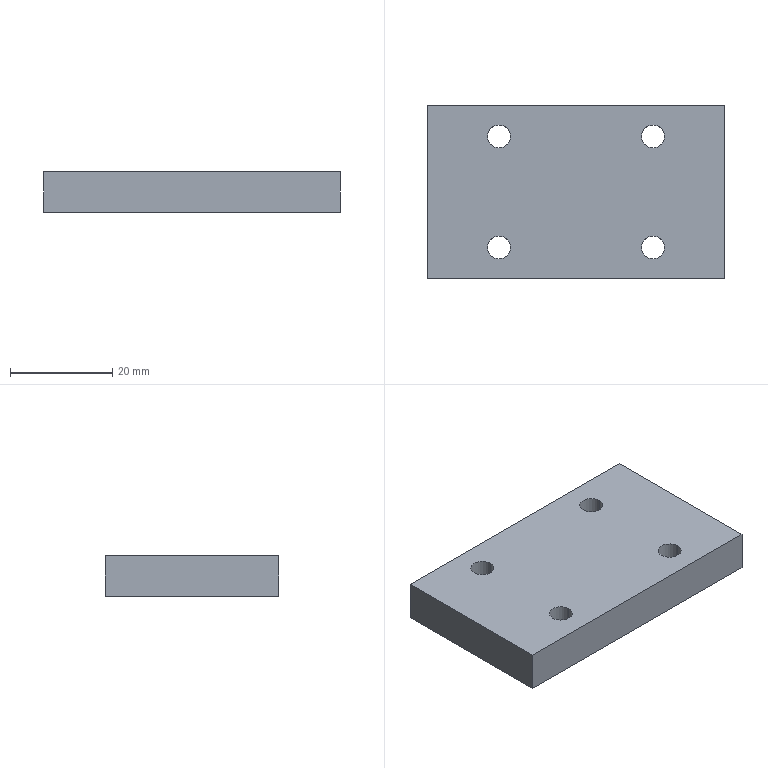Part | SolidWorks | features BaseBody 1 | 1 solid | 14 faces | box 58 x 34 x 8 mm | volume 15267 mm3 | cylinder 8 | plane 6 | commonest cylinder face diameters 4.5 x8
STEP:
#1=CARTESIAN_POINT('',(12.83,10.88,28.));
#2=VERTEX_POINT('',#1);
#3=CARTESIAN_POINT('',(17.33,10.88,28.));
#4=VERTEX_POINT('',#3);
#5=CARTESIAN_POINT('',(15.08,10.88,28.));
#6=DIRECTION('',(0.,0.,1.));
#7=DIRECTION('',(1.,0.,0.));
#8=AXIS2_PLACEMENT_3D('',#5,#6,#7);
#9=CIRCLE('',#8,2.25);
#10=EDGE_CURVE('',#2,#4,#9,.T.);
#11=ORIENTED_EDGE('',*,*,#10,.F.);
#12=CARTESIAN_POINT('',(12.83,10.88,36.));
#13=VERTEX_POINT('',#12);
#14=CARTESIAN_POINT('',(12.83,10.88,27.));
#15=DIRECTION('',(0.,0.,1.));
#16=VECTOR('',#15,1000.);
#17=LINE('',#14,#16);
#18=EDGE_CURVE('',#2,#13,#17,.T.);
#19=ORIENTED_EDGE('',*,*,#18,.T.);
#20=CARTESIAN_POINT('',(17.33,10.88,36.));
#21=VERTEX_POINT('',#20);
#22=CARTESIAN_POINT('',(15.08,10.88,36.));
#23=DIRECTION('',(0.,0.,-1.));
#24=DIRECTION('',(1.,0.,0.));
#25=AXIS2_PLACEMENT_3D('',#22,#23,#24);
#26=CIRCLE('',#25,2.25);
#27=EDGE_CURVE('',#21,#13,#26,.T.);
#28=ORIENTED_EDGE('',*,*,#27,.F.);
#29=CARTESIAN_POINT('',(17.33,10.88,27.));
#30=DIRECTION('',(0.,0.,1.));
#31=VECTOR('',#30,1000.);
#32=LINE('',#29,#31);
#33=EDGE_CURVE('',#4,#21,#32,.T.);
#34=ORIENTED_EDGE('',*,*,#33,.F.);
#35=EDGE_LOOP('',(#11,#19,#28,#34));
#36=FACE_OUTER_BOUND('',#35,.T.);
#37=CARTESIAN_POINT('',(15.08,10.88,27.));
#38=DIRECTION('',(0.,0.,1.));
#39=DIRECTION('',(1.,0.,0.));
#40=AXIS2_PLACEMENT_3D('',#37,#38,#39);
#41=CYLINDRICAL_SURFACE('',#40,2.25);
#42=ADVANCED_FACE('',(#36),#41,.F.);
#43=CARTESIAN_POINT('',(-17.33,10.88,28.));
#44=VERTEX_POINT('',#43);
#45=CARTESIAN_POINT('',(-12.83,10.88,28.));
#46=VERTEX_POINT('',#45);
#47=CARTESIAN_POINT('',(-15.08,10.88,28.));
#48=DIRECTION('',(0.,0.,1.));
#49=DIRECTION('',(1.,0.,0.));
#50=AXIS2_PLACEMENT_3D('',#47,#48,#49);
#51=CIRCLE('',#50,2.25);
#52=EDGE_CURVE('',#44,#46,#51,.T.);
#53=ORIENTED_EDGE('',*,*,#52,.F.);
#54=CARTESIAN_POINT('',(-17.33,10.88,36.));
#55=VERTEX_POINT('',#54);
#56=CARTESIAN_POINT('',(-17.33,10.88,27.));
#57=DIRECTION('',(0.,0.,1.));
#58=VECTOR('',#57,1000.);
#59=LINE('',#56,#58);
#60=EDGE_CURVE('',#44,#55,#59,.T.);
#61=ORIENTED_EDGE('',*,*,#60,.T.);
#62=CARTESIAN_POINT('',(-12.83,10.88,36.));
#63=VERTEX_POINT('',#62);
#64=CARTESIAN_POINT('',(-15.08,10.88,36.));
#65=DIRECTION('',(0.,0.,-1.));
#66=DIRECTION('',(1.,0.,0.));
#67=AXIS2_PLACEMENT_3D('',#64,#65,#66);
#68=CIRCLE('',#67,2.25);
#69=EDGE_CURVE('',#63,#55,#68,.T.);
#70=ORIENTED_EDGE('',*,*,#69,.F.);
#71=CARTESIAN_POINT('',(-12.83,10.88,27.));
#72=DIRECTION('',(0.,0.,1.));
#73=VECTOR('',#72,1000.);
#74=LINE('',#71,#73);
#75=EDGE_CURVE('',#46,#63,#74,.T.);
#76=ORIENTED_EDGE('',*,*,#75,.F.);
#77=EDGE_LOOP('',(#53,#61,#70,#76));
#78=FACE_OUTER_BOUND('',#77,.T.);
#79=CARTESIAN_POINT('',(-15.08,10.88,27.));
#80=DIRECTION('',(0.,0.,1.));
#81=DIRECTION('',(1.,0.,0.));
#82=AXIS2_PLACEMENT_3D('',#79,#80,#81);
#83=CYLINDRICAL_SURFACE('',#82,2.25);
#84=ADVANCED_FACE('',(#78),#83,.F.);
#85=CARTESIAN_POINT('',(12.83,-10.88,28.));
#86=VERTEX_POINT('',#85);
#87=CARTESIAN_POINT('',(17.33,-10.88,28.));
#88=VERTEX_POINT('',#87);
#89=CARTESIAN_POINT('',(15.08,-10.88,28.));
#90=DIRECTION('',(0.,0.,1.));
#91=DIRECTION('',(1.,0.,0.));
#92=AXIS2_PLACEMENT_3D('',#89,#90,#91);
#93=CIRCLE('',#92,2.25);
#94=EDGE_CURVE('',#86,#88,#93,.T.);
#95=ORIENTED_EDGE('',*,*,#94,.F.);
#96=CARTESIAN_POINT('',(12.83,-10.88,36.));
#97=VERTEX_POINT('',#96);
#98=CARTESIAN_POINT('',(12.83,-10.88,27.));
#99=DIRECTION('',(0.,0.,1.));
#100=VECTOR('',#99,1000.);
#101=LINE('',#98,#100);
#102=EDGE_CURVE('',#86,#97,#101,.T.);
#103=ORIENTED_EDGE('',*,*,#102,.T.);
#104=CARTESIAN_POINT('',(17.33,-10.88,36.));
#105=VERTEX_POINT('',#104);
#106=CARTESIAN_POINT('',(15.08,-10.88,36.));
#107=DIRECTION('',(0.,0.,-1.));
#108=DIRECTION('',(1.,0.,0.));
#109=AXIS2_PLACEMENT_3D('',#106,#107,#108);
#110=CIRCLE('',#109,2.25);
#111=EDGE_CURVE('',#105,#97,#110,.T.);
#112=ORIENTED_EDGE('',*,*,#111,.F.);
#113=CARTESIAN_POINT('',(17.33,-10.88,27.));
#114=DIRECTION('',(0.,0.,1.));
#115=VECTOR('',#114,1000.);
#116=LINE('',#113,#115);
#117=EDGE_CURVE('',#88,#105,#116,.T.);
#118=ORIENTED_EDGE('',*,*,#117,.F.);
#119=EDGE_LOOP('',(#95,#103,#112,#118));
#120=FACE_OUTER_BOUND('',#119,.T.);
#121=CARTESIAN_POINT('',(15.08,-10.88,27.));
#122=DIRECTION('',(0.,0.,1.));
#123=DIRECTION('',(1.,0.,0.));
#124=AXIS2_PLACEMENT_3D('',#121,#122,#123);
#125=CYLINDRICAL_SURFACE('',#124,2.25);
#126=ADVANCED_FACE('',(#120),#125,.F.);
#127=CARTESIAN_POINT('',(-17.33,-10.88,28.));
#128=VERTEX_POINT('',#127);
#129=CARTESIAN_POINT('',(-12.83,-10.88,28.));
#130=VERTEX_POINT('',#129);
#131=CARTESIAN_POINT('',(-15.08,-10.88,28.));
#132=DIRECTION('',(0.,0.,1.));
#133=DIRECTION('',(1.,0.,0.));
#134=AXIS2_PLACEMENT_3D('',#131,#132,#133);
#135=CIRCLE('',#134,2.25);
#136=EDGE_CURVE('',#128,#130,#135,.T.);
#137=ORIENTED_EDGE('',*,*,#136,.F.);
#138=CARTESIAN_POINT('',(-17.33,-10.88,36.));
#139=VERTEX_POINT('',#138);
#140=CARTESIAN_POINT('',(-17.33,-10.88,27.));
#141=DIRECTION('',(0.,0.,1.));
#142=VECTOR('',#141,1000.);
#143=LINE('',#140,#142);
#144=EDGE_CURVE('',#128,#139,#143,.T.);
#145=ORIENTED_EDGE('',*,*,#144,.T.);
#146=CARTESIAN_POINT('',(-12.83,-10.88,36.));
#147=VERTEX_POINT('',#146);
#148=CARTESIAN_POINT('',(-15.08,-10.88,36.));
#149=DIRECTION('',(0.,0.,-1.));
#150=DIRECTION('',(1.,0.,0.));
#151=AXIS2_PLACEMENT_3D('',#148,#149,#150);
#152=CIRCLE('',#151,2.25);
#153=EDGE_CURVE('',#147,#139,#152,.T.);
#154=ORIENTED_EDGE('',*,*,#153,.F.);
#155=CARTESIAN_POINT('',(-12.83,-10.88,27.));
#156=DIRECTION('',(0.,0.,1.));
#157=VECTOR('',#156,1000.);
#158=LINE('',#155,#157);
#159=EDGE_CURVE('',#130,#147,#158,.T.);
#160=ORIENTED_EDGE('',*,*,#159,.F.);
#161=EDGE_LOOP('',(#137,#145,#154,#160));
#162=FACE_OUTER_BOUND('',#161,.T.);
#163=CARTESIAN_POINT('',(-15.08,-10.88,27.));
#164=DIRECTION('',(0.,0.,1.));
#165=DIRECTION('',(1.,0.,0.));
#166=AXIS2_PLACEMENT_3D('',#163,#164,#165);
#167=CYLINDRICAL_SURFACE('',#166,2.25);
#168=ADVANCED_FACE('',(#162),#167,.F.);
#169=ORIENTED_EDGE('',*,*,#27,.T.);
#170=CARTESIAN_POINT('',(15.08,10.88,36.));
#171=DIRECTION('',(0.,0.,-1.));
#172=DIRECTION('',(1.,0.,0.));
#173=AXIS2_PLACEMENT_3D('',#170,#171,#172);
#174=CIRCLE('',#173,2.25);
#175=EDGE_CURVE('',#13,#21,#174,.T.);
#176=ORIENTED_EDGE('',*,*,#175,.T.);
#177=EDGE_LOOP('',(#169,#176));
#178=FACE_BOUND('',#177,.T.);
#179=ORIENTED_EDGE('',*,*,#69,.T.);
#180=CARTESIAN_POINT('',(-15.08,10.88,36.));
#181=DIRECTION('',(0.,0.,-1.));
#182=DIRECTION('',(1.,0.,0.));
#183=AXIS2_PLACEMENT_3D('',#180,#181,#182);
#184=CIRCLE('',#183,2.25);
#185=EDGE_CURVE('',#55,#63,#184,.T.);
#186=ORIENTED_EDGE('',*,*,#185,.T.);
#187=EDGE_LOOP('',(#179,#186));
#188=FACE_BOUND('',#187,.T.);
#189=ORIENTED_EDGE('',*,*,#111,.T.);
#190=CARTESIAN_POINT('',(15.08,-10.88,36.));
#191=DIRECTION('',(0.,0.,-1.));
#192=DIRECTION('',(1.,0.,0.));
#193=AXIS2_PLACEMENT_3D('',#190,#191,#192);
#194=CIRCLE('',#193,2.25);
#195=EDGE_CURVE('',#97,#105,#194,.T.);
#196=ORIENTED_EDGE('',*,*,#195,.T.);
#197=EDGE_LOOP('',(#189,#196));
#198=FACE_BOUND('',#197,.T.);
#199=ORIENTED_EDGE('',*,*,#153,.T.);
#200=CARTESIAN_POINT('',(-15.08,-10.88,36.));
#201=DIRECTION('',(0.,0.,-1.));
#202=DIRECTION('',(1.,0.,0.));
#203=AXIS2_PLACEMENT_3D('',#200,#201,#202);
#204=CIRCLE('',#203,2.25);
#205=EDGE_CURVE('',#139,#147,#204,.T.);
#206=ORIENTED_EDGE('',*,*,#205,.T.);
#207=EDGE_LOOP('',(#199,#206));
#208=FACE_BOUND('',#207,.T.);
#209=CARTESIAN_POINT('',(29.,-17.,36.));
#210=VERTEX_POINT('',#209);
#211=CARTESIAN_POINT('',(29.,17.,36.));
#212=VERTEX_POINT('',#211);
#213=CARTESIAN_POINT('',(29.,-17.,36.));
#214=DIRECTION('',(0.,1.,0.));
#215=VECTOR('',#214,1000.);
#216=LINE('',#213,#215);
#217=EDGE_CURVE('',#210,#212,#216,.T.);
#218=ORIENTED_EDGE('',*,*,#217,.T.);
#219=CARTESIAN_POINT('',(-29.,17.,36.));
#220=VERTEX_POINT('',#219);
#221=CARTESIAN_POINT('',(-29.,17.,36.));
#222=DIRECTION('',(-1.,0.,0.));
#223=VECTOR('',#222,1000.);
#224=LINE('',#221,#223);
#225=EDGE_CURVE('',#212,#220,#224,.T.);
#226=ORIENTED_EDGE('',*,*,#225,.T.);
#227=CARTESIAN_POINT('',(-29.,-17.,36.));
#228=VERTEX_POINT('',#227);
#229=CARTESIAN_POINT('',(-29.,-17.,36.));
#230=DIRECTION('',(0.,-1.,0.));
#231=VECTOR('',#230,1000.);
#232=LINE('',#229,#231);
#233=EDGE_CURVE('',#220,#228,#232,.T.);
#234=ORIENTED_EDGE('',*,*,#233,.T.);
#235=CARTESIAN_POINT('',(-29.,-17.,36.));
#236=DIRECTION('',(1.,0.,0.));
#237=VECTOR('',#236,1000.);
#238=LINE('',#235,#237);
#239=EDGE_CURVE('',#228,#210,#238,.T.);
#240=ORIENTED_EDGE('',*,*,#239,.T.);
#241=EDGE_LOOP('',(#218,#226,#234,#240));
#242=FACE_OUTER_BOUND('',#241,.T.);
#243=CARTESIAN_POINT('',(-29.,-17.,36.));
#244=DIRECTION('',(0.,0.,1.));
#245=DIRECTION('',(1.,0.,0.));
#246=AXIS2_PLACEMENT_3D('',#243,#244,#245);
#247=PLANE('',#246);
#248=ADVANCED_FACE('',(#178,#188,#198,#208,#242),#247,.T.);
#249=ORIENTED_EDGE('',*,*,#18,.F.);
#250=CARTESIAN_POINT('',(15.08,10.88,28.));
#251=DIRECTION('',(0.,0.,1.));
#252=DIRECTION('',(1.,0.,0.));
#253=AXIS2_PLACEMENT_3D('',#250,#251,#252);
#254=CIRCLE('',#253,2.25);
#255=EDGE_CURVE('',#4,#2,#254,.T.);
#256=ORIENTED_EDGE('',*,*,#255,.F.);
#257=ORIENTED_EDGE('',*,*,#33,.T.);
#258=ORIENTED_EDGE('',*,*,#175,.F.);
#259=EDGE_LOOP('',(#249,#256,#257,#258));
#260=FACE_OUTER_BOUND('',#259,.T.);
#261=CARTESIAN_POINT('',(15.08,10.88,27.));
#262=DIRECTION('',(0.,0.,1.));
#263=DIRECTION('',(1.,0.,0.));
#264=AXIS2_PLACEMENT_3D('',#261,#262,#263);
#265=CYLINDRICAL_SURFACE('',#264,2.25);
#266=ADVANCED_FACE('',(#260),#265,.F.);
#267=ORIENTED_EDGE('',*,*,#60,.F.);
#268=CARTESIAN_POINT('',(-15.08,10.88,28.));
#269=DIRECTION('',(0.,0.,1.));
#270=DIRECTION('',(1.,0.,0.));
#271=AXIS2_PLACEMENT_3D('',#268,#269,#270);
#272=CIRCLE('',#271,2.25);
#273=EDGE_CURVE('',#46,#44,#272,.T.);
#274=ORIENTED_EDGE('',*,*,#273,.F.);
#275=ORIENTED_EDGE('',*,*,#75,.T.);
#276=ORIENTED_EDGE('',*,*,#185,.F.);
#277=EDGE_LOOP('',(#267,#274,#275,#276));
#278=FACE_OUTER_BOUND('',#277,.T.);
#279=CARTESIAN_POINT('',(-15.08,10.88,27.));
#280=DIRECTION('',(0.,0.,1.));
#281=DIRECTION('',(1.,0.,0.));
#282=AXIS2_PLACEMENT_3D('',#279,#280,#281);
#283=CYLINDRICAL_SURFACE('',#282,2.25);
#284=ADVANCED_FACE('',(#278),#283,.F.);
#285=ORIENTED_EDGE('',*,*,#102,.F.);
#286=CARTESIAN_POINT('',(15.08,-10.88,28.));
#287=DIRECTION('',(0.,0.,1.));
#288=DIRECTION('',(1.,0.,0.));
#289=AXIS2_PLACEMENT_3D('',#286,#287,#288);
#290=CIRCLE('',#289,2.25);
#291=EDGE_CURVE('',#88,#86,#290,.T.);
#292=ORIENTED_EDGE('',*,*,#291,.F.);
#293=ORIENTED_EDGE('',*,*,#117,.T.);
#294=ORIENTED_EDGE('',*,*,#195,.F.);
#295=EDGE_LOOP('',(#285,#292,#293,#294));
#296=FACE_OUTER_BOUND('',#295,.T.);
#297=CARTESIAN_POINT('',(15.08,-10.88,27.));
#298=DIRECTION('',(0.,0.,1.));
#299=DIRECTION('',(1.,0.,0.));
#300=AXIS2_PLACEMENT_3D('',#297,#298,#299);
#301=CYLINDRICAL_SURFACE('',#300,2.25);
#302=ADVANCED_FACE('',(#296),#301,.F.);
#303=ORIENTED_EDGE('',*,*,#144,.F.);
#304=CARTESIAN_POINT('',(-15.08,-10.88,28.));
#305=DIRECTION('',(0.,0.,1.));
#306=DIRECTION('',(1.,0.,0.));
#307=AXIS2_PLACEMENT_3D('',#304,#305,#306);
#308=CIRCLE('',#307,2.25);
#309=EDGE_CURVE('',#130,#128,#308,.T.);
#310=ORIENTED_EDGE('',*,*,#309,.F.);
#311=ORIENTED_EDGE('',*,*,#159,.T.);
#312=ORIENTED_EDGE('',*,*,#205,.F.);
#313=EDGE_LOOP('',(#303,#310,#311,#312));
#314=FACE_OUTER_BOUND('',#313,.T.);
#315=CARTESIAN_POINT('',(-15.08,-10.88,27.));
#316=DIRECTION('',(0.,0.,1.));
#317=DIRECTION('',(1.,0.,0.));
#318=AXIS2_PLACEMENT_3D('',#315,#316,#317);
#319=CYLINDRICAL_SURFACE('',#318,2.25);
#320=ADVANCED_FACE('',(#314),#319,.F.);
#321=ORIENTED_EDGE('',*,*,#225,.F.);
#322=CARTESIAN_POINT('',(29.,17.,28.));
#323=VERTEX_POINT('',#322);
#324=CARTESIAN_POINT('',(29.,17.,28.));
#325=DIRECTION('',(0.,0.,-1.));
#326=VECTOR('',#325,1000.);
#327=LINE('',#324,#326);
#328=EDGE_CURVE('',#212,#323,#327,.T.);
#329=ORIENTED_EDGE('',*,*,#328,.T.);
#330=CARTESIAN_POINT('',(-29.,17.,28.));
#331=VERTEX_POINT('',#330);
#332=CARTESIAN_POINT('',(-29.,17.,28.));
#333=DIRECTION('',(-1.,0.,0.));
#334=VECTOR('',#333,1000.);
#335=LINE('',#332,#334);
#336=EDGE_CURVE('',#323,#331,#335,.T.);
#337=ORIENTED_EDGE('',*,*,#336,.T.);
#338=CARTESIAN_POINT('',(-29.,17.,28.));
#339=DIRECTION('',(0.,0.,1.));
#340=VECTOR('',#339,1000.);
#341=LINE('',#338,#340);
#342=EDGE_CURVE('',#331,#220,#341,.T.);
#343=ORIENTED_EDGE('',*,*,#342,.T.);
#344=EDGE_LOOP('',(#321,#329,#337,#343));
#345=FACE_OUTER_BOUND('',#344,.T.);
#346=CARTESIAN_POINT('',(-29.,17.,28.));
#347=DIRECTION('',(0.,1.,0.));
#348=DIRECTION('',(0.,0.,1.));
#349=AXIS2_PLACEMENT_3D('',#346,#347,#348);
#350=PLANE('',#349);
#351=ADVANCED_FACE('',(#345),#350,.T.);
#352=ORIENTED_EDGE('',*,*,#328,.F.);
#353=ORIENTED_EDGE('',*,*,#217,.F.);
#354=CARTESIAN_POINT('',(29.,-17.,28.));
#355=VERTEX_POINT('',#354);
#356=CARTESIAN_POINT('',(29.,-17.,28.));
#357=DIRECTION('',(0.,0.,-1.));
#358=VECTOR('',#357,1000.);
#359=LINE('',#356,#358);
#360=EDGE_CURVE('',#210,#355,#359,.T.);
#361=ORIENTED_EDGE('',*,*,#360,.T.);
#362=CARTESIAN_POINT('',(29.,-17.,28.));
#363=DIRECTION('',(0.,1.,0.));
#364=VECTOR('',#363,1000.);
#365=LINE('',#362,#364);
#366=EDGE_CURVE('',#355,#323,#365,.T.);
#367=ORIENTED_EDGE('',*,*,#366,.T.);
#368=EDGE_LOOP('',(#352,#353,#361,#367));
#369=FACE_OUTER_BOUND('',#368,.T.);
#370=CARTESIAN_POINT('',(29.,-17.,28.));
#371=DIRECTION('',(1.,0.,0.));
#372=DIRECTION('',(0.,0.,-1.));
#373=AXIS2_PLACEMENT_3D('',#370,#371,#372);
#374=PLANE('',#373);
#375=ADVANCED_FACE('',(#369),#374,.T.);
#376=ORIENTED_EDGE('',*,*,#239,.F.);
#377=CARTESIAN_POINT('',(-29.,-17.,28.));
#378=VERTEX_POINT('',#377);
#379=CARTESIAN_POINT('',(-29.,-17.,28.));
#380=DIRECTION('',(0.,0.,1.));
#381=VECTOR('',#380,1000.);
#382=LINE('',#379,#381);
#383=EDGE_CURVE('',#378,#228,#382,.T.);
#384=ORIENTED_EDGE('',*,*,#383,.F.);
#385=CARTESIAN_POINT('',(-29.,-17.,28.));
#386=DIRECTION('',(-1.,0.,0.));
#387=VECTOR('',#386,1000.);
#388=LINE('',#385,#387);
#389=EDGE_CURVE('',#355,#378,#388,.T.);
#390=ORIENTED_EDGE('',*,*,#389,.F.);
#391=ORIENTED_EDGE('',*,*,#360,.F.);
#392=EDGE_LOOP('',(#376,#384,#390,#391));
#393=FACE_OUTER_BOUND('',#392,.T.);
#394=CARTESIAN_POINT('',(-29.,-17.,28.));
#395=DIRECTION('',(0.,1.,0.));
#396=DIRECTION('',(0.,0.,1.));
#397=AXIS2_PLACEMENT_3D('',#394,#395,#396);
#398=PLANE('',#397);
#399=ADVANCED_FACE('',(#393),#398,.F.);
#400=ORIENTED_EDGE('',*,*,#342,.F.);
#401=CARTESIAN_POINT('',(-29.,-17.,28.));
#402=DIRECTION('',(0.,1.,0.));
#403=VECTOR('',#402,1000.);
#404=LINE('',#401,#403);
#405=EDGE_CURVE('',#378,#331,#404,.T.);
#406=ORIENTED_EDGE('',*,*,#405,.F.);
#407=ORIENTED_EDGE('',*,*,#383,.T.);
#408=ORIENTED_EDGE('',*,*,#233,.F.);
#409=EDGE_LOOP('',(#400,#406,#407,#408));
#410=FACE_OUTER_BOUND('',#409,.T.);
#411=CARTESIAN_POINT('',(-29.,-17.,28.));
#412=DIRECTION('',(1.,0.,0.));
#413=DIRECTION('',(0.,0.,-1.));
#414=AXIS2_PLACEMENT_3D('',#411,#412,#413);
#415=PLANE('',#414);
#416=ADVANCED_FACE('',(#410),#415,.F.);
#417=ORIENTED_EDGE('',*,*,#255,.T.);
#418=ORIENTED_EDGE('',*,*,#10,.T.);
#419=EDGE_LOOP('',(#417,#418));
#420=FACE_BOUND('',#419,.T.);
#421=ORIENTED_EDGE('',*,*,#273,.T.);
#422=ORIENTED_EDGE('',*,*,#52,.T.);
#423=EDGE_LOOP('',(#421,#422));
#424=FACE_BOUND('',#423,.T.);
#425=ORIENTED_EDGE('',*,*,#291,.T.);
#426=ORIENTED_EDGE('',*,*,#94,.T.);
#427=EDGE_LOOP('',(#425,#426));
#428=FACE_BOUND('',#427,.T.);
#429=ORIENTED_EDGE('',*,*,#309,.T.);
#430=ORIENTED_EDGE('',*,*,#136,.T.);
#431=EDGE_LOOP('',(#429,#430));
#432=FACE_BOUND('',#431,.T.);
#433=ORIENTED_EDGE('',*,*,#366,.F.);
#434=ORIENTED_EDGE('',*,*,#389,.T.);
#435=ORIENTED_EDGE('',*,*,#405,.T.);
#436=ORIENTED_EDGE('',*,*,#336,.F.);
#437=EDGE_LOOP('',(#433,#434,#435,#436));
#438=FACE_OUTER_BOUND('',#437,.T.);
#439=CARTESIAN_POINT('',(-29.,-17.,28.));
#440=DIRECTION('',(0.,0.,1.));
#441=DIRECTION('',(1.,0.,0.));
#442=AXIS2_PLACEMENT_3D('',#439,#440,#441);
#443=PLANE('',#442);
#444=ADVANCED_FACE('',(#420,#424,#428,#432,#438),#443,.F.);
#445=CLOSED_SHELL('',(#42,#84,#126,#168,#248,#266,#284,#302,#320,#351,#375,#399,#416,#444));
#446=MANIFOLD_SOLID_BREP('',#445);
#447=CARTESIAN_POINT('',(0.,0.,0.));
#448=DIRECTION('',(0.,0.,1.));
#449=DIRECTION('',(1.,0.,0.));
#450=AXIS2_PLACEMENT_3D('',#447,#448,#449);
#451=(LENGTH_UNIT()NAMED_UNIT(*)SI_UNIT(.MILLI.,.METRE.));
#452=UNCERTAINTY_MEASURE_WITH_UNIT(LENGTH_MEASURE(0.00001),#451,'','');
#453=(NAMED_UNIT(*)PLANE_ANGLE_UNIT()SI_UNIT($,.RADIAN.));
#454=(NAMED_UNIT(*)SI_UNIT($,.STERADIAN.)SOLID_ANGLE_UNIT());
#455=(GEOMETRIC_REPRESENTATION_CONTEXT(3)GLOBAL_UNCERTAINTY_ASSIGNED_CONTEXT((#452))GLOBAL_UNIT_ASSIGNED_CONTEXT((#451,#453,#454))REPRESENTATION_CONTEXT('',''));
#456=ADVANCED_BREP_SHAPE_REPRESENTATION('',(#446,#450),#455);